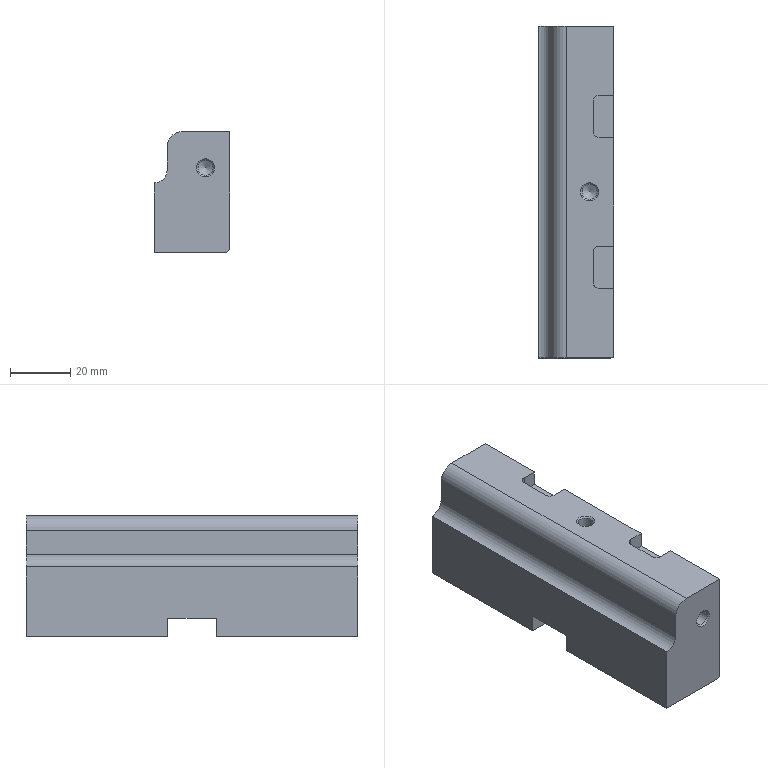Part | STEP file | gslz 2016.10.28-6_id746_x_t | 1 solid | 42 faces | box 25 x 110 x 40 mm | volume 96354 mm3 | plane 21 | cylinder 11 | cone 10 | commonest cylinder face diameters 4 x4 5 x3 6.8 x2 8.5 x1 10 x1
STEP:
#1=CARTESIAN_POINT('',(115.2,175.,53.));
#2=VERTEX_POINT('',#1);
#3=CARTESIAN_POINT('',(115.2,175.,57.));
#4=DIRECTION('',(1.,0.,0.));
#5=DIRECTION('',(0.,0.,-1.));
#6=AXIS2_PLACEMENT_3D('',#3,#4,#5);
#7=CIRCLE('',#6,4.);
#8=EDGE_CURVE('',#2,#2,#7,.T.);
#9=ORIENTED_EDGE('',*,*,#8,.F.);
#10=EDGE_LOOP('',(#9));
#11=FACE_BOUND('',#10,.T.);
#12=CARTESIAN_POINT('',(115.2,158.,40.));
#13=VERTEX_POINT('',#12);
#14=CARTESIAN_POINT('',(115.2,158.,45.));
#15=VERTEX_POINT('',#14);
#16=CARTESIAN_POINT('',(115.2,158.,35.));
#17=DIRECTION('',(0.,0.,1.));
#18=VECTOR('',#17,1.);
#19=LINE('',#16,#18);
#20=EDGE_CURVE('',#13,#15,#19,.T.);
#21=ORIENTED_EDGE('',*,*,#20,.F.);
#22=CARTESIAN_POINT('',(115.2,205.01,40.));
#23=VERTEX_POINT('',#22);
#24=CARTESIAN_POINT('',(115.2,930.778,40.));
#25=DIRECTION('',(0.,1.,0.));
#26=VECTOR('',#25,1.);
#27=LINE('',#24,#26);
#28=EDGE_CURVE('',#13,#23,#27,.T.);
#29=ORIENTED_EDGE('',*,*,#28,.T.);
#30=CARTESIAN_POINT('',(115.2,205.01,79.));
#31=VERTEX_POINT('',#30);
#32=CARTESIAN_POINT('',(115.2,205.01,79.));
#33=DIRECTION('',(0.,0.,-1.));
#34=VECTOR('',#33,1.);
#35=LINE('',#32,#34);
#36=EDGE_CURVE('',#31,#23,#35,.T.);
#37=ORIENTED_EDGE('',*,*,#36,.F.);
#38=CARTESIAN_POINT('',(115.2,182.,79.));
#39=VERTEX_POINT('',#38);
#40=CARTESIAN_POINT('',(115.2,101.,79.));
#41=DIRECTION('',(0.,1.,0.));
#42=VECTOR('',#41,1.);
#43=LINE('',#40,#42);
#44=EDGE_CURVE('',#39,#31,#43,.T.);
#45=ORIENTED_EDGE('',*,*,#44,.F.);
#46=CARTESIAN_POINT('',(115.2,182.,74.));
#47=VERTEX_POINT('',#46);
#48=CARTESIAN_POINT('',(115.2,182.,49.));
#49=DIRECTION('',(0.,-0.000000014,-1.));
#50=VECTOR('',#49,1.);
#51=LINE('',#48,#50);
#52=EDGE_CURVE('',#39,#47,#51,.T.);
#53=ORIENTED_EDGE('',*,*,#52,.T.);
#54=CARTESIAN_POINT('',(115.2,168.,74.));
#55=VERTEX_POINT('',#54);
#56=CARTESIAN_POINT('',(115.2,932.793,74.));
#57=DIRECTION('',(0.,1.,0.000000015));
#58=VECTOR('',#57,1.);
#59=LINE('',#56,#58);
#60=EDGE_CURVE('',#55,#47,#59,.T.);
#61=ORIENTED_EDGE('',*,*,#60,.F.);
#62=CARTESIAN_POINT('',(115.2,168.,79.));
#63=VERTEX_POINT('',#62);
#64=CARTESIAN_POINT('',(115.2,168.,49.));
#65=DIRECTION('',(0.,-0.000000014,-1.));
#66=VECTOR('',#65,1.);
#67=LINE('',#64,#66);
#68=EDGE_CURVE('',#63,#55,#67,.T.);
#69=ORIENTED_EDGE('',*,*,#68,.F.);
#70=CARTESIAN_POINT('',(115.2,132.,79.));
#71=VERTEX_POINT('',#70);
#72=CARTESIAN_POINT('',(115.2,101.,79.));
#73=DIRECTION('',(0.,1.,0.));
#74=VECTOR('',#73,1.);
#75=LINE('',#72,#74);
#76=EDGE_CURVE('',#71,#63,#75,.T.);
#77=ORIENTED_EDGE('',*,*,#76,.F.);
#78=CARTESIAN_POINT('',(115.2,132.,74.));
#79=VERTEX_POINT('',#78);
#80=CARTESIAN_POINT('',(115.2,132.,49.));
#81=DIRECTION('',(0.,-0.000000014,-1.));
#82=VECTOR('',#81,1.);
#83=LINE('',#80,#82);
#84=EDGE_CURVE('',#71,#79,#83,.T.);
#85=ORIENTED_EDGE('',*,*,#84,.T.);
#86=CARTESIAN_POINT('',(115.2,118.,74.));
#87=VERTEX_POINT('',#86);
#88=CARTESIAN_POINT('',(115.2,928.763,74.));
#89=DIRECTION('',(0.,1.,-0.000000015));
#90=VECTOR('',#89,1.);
#91=LINE('',#88,#90);
#92=EDGE_CURVE('',#87,#79,#91,.T.);
#93=ORIENTED_EDGE('',*,*,#92,.F.);
#94=CARTESIAN_POINT('',(115.2,118.,79.));
#95=VERTEX_POINT('',#94);
#96=CARTESIAN_POINT('',(115.2,118.,49.));
#97=DIRECTION('',(0.,-0.000000014,-1.));
#98=VECTOR('',#97,1.);
#99=LINE('',#96,#98);
#100=EDGE_CURVE('',#95,#87,#99,.T.);
#101=ORIENTED_EDGE('',*,*,#100,.F.);
#102=CARTESIAN_POINT('',(115.2,95.01,79.));
#103=VERTEX_POINT('',#102);
#104=CARTESIAN_POINT('',(115.2,101.,79.));
#105=DIRECTION('',(0.,1.,0.));
#106=VECTOR('',#105,1.);
#107=LINE('',#104,#106);
#108=EDGE_CURVE('',#103,#95,#107,.T.);
#109=ORIENTED_EDGE('',*,*,#108,.F.);
#110=CARTESIAN_POINT('',(115.2,95.01,40.));
#111=VERTEX_POINT('',#110);
#112=CARTESIAN_POINT('',(115.2,95.01,79.));
#113=DIRECTION('',(0.,0.,1.));
#114=VECTOR('',#113,1.);
#115=LINE('',#112,#114);
#116=EDGE_CURVE('',#111,#103,#115,.T.);
#117=ORIENTED_EDGE('',*,*,#116,.F.);
#118=CARTESIAN_POINT('',(115.2,142.,40.));
#119=VERTEX_POINT('',#118);
#120=CARTESIAN_POINT('',(115.2,930.778,40.));
#121=DIRECTION('',(0.,1.,0.));
#122=VECTOR('',#121,1.);
#123=LINE('',#120,#122);
#124=EDGE_CURVE('',#111,#119,#123,.T.);
#125=ORIENTED_EDGE('',*,*,#124,.T.);
#126=CARTESIAN_POINT('',(115.2,142.,45.));
#127=VERTEX_POINT('',#126);
#128=CARTESIAN_POINT('',(115.2,142.,46.));
#129=DIRECTION('',(0.,0.,1.));
#130=VECTOR('',#129,1.);
#131=LINE('',#128,#130);
#132=EDGE_CURVE('',#119,#127,#131,.T.);
#133=ORIENTED_EDGE('',*,*,#132,.T.);
#134=CARTESIAN_POINT('',(115.2,930.778,45.));
#135=DIRECTION('',(0.,1.,0.));
#136=VECTOR('',#135,1.);
#137=LINE('',#134,#136);
#138=EDGE_CURVE('',#127,#15,#137,.T.);
#139=ORIENTED_EDGE('',*,*,#138,.T.);
#140=EDGE_LOOP('',(#21,#29,#37,#45,#53,#61,#69,#77,#85,#93,#101,#109,#117,#125,#133,#139));
#141=FACE_BOUND('',#140,.T.);
#142=CARTESIAN_POINT('',(115.2,125.,53.));
#143=VERTEX_POINT('',#142);
#144=CARTESIAN_POINT('',(115.2,125.,57.));
#145=DIRECTION('',(1.,0.,0.));
#146=DIRECTION('',(0.,0.,-1.));
#147=AXIS2_PLACEMENT_3D('',#144,#145,#146);
#148=CIRCLE('',#147,4.);
#149=EDGE_CURVE('',#143,#143,#148,.T.);
#150=ORIENTED_EDGE('',*,*,#149,.F.);
#151=EDGE_LOOP('',(#150));
#152=FACE_BOUND('',#151,.T.);
#153=CARTESIAN_POINT('',(115.2,930.778,49.));
#154=DIRECTION('',(-1.,0.,0.));
#155=DIRECTION('',(0.,0.,1.));
#156=AXIS2_PLACEMENT_3D('',#153,#154,#155);
#157=PLANE('',#156);
#158=ADVANCED_FACE('',(#11,#141,#152),#157,.F.);
#159=CARTESIAN_POINT('',(114.2,95.01,39.));
#160=VERTEX_POINT('',#159);
#161=CARTESIAN_POINT('',(90.2,95.01,39.));
#162=VERTEX_POINT('',#161);
#163=CARTESIAN_POINT('',(100.2,95.01,39.));
#164=DIRECTION('',(-1.,0.,0.));
#165=VECTOR('',#164,1.);
#166=LINE('',#163,#165);
#167=EDGE_CURVE('',#160,#162,#166,.T.);
#168=ORIENTED_EDGE('',*,*,#167,.F.);
#169=CARTESIAN_POINT('',(127.2,95.01,52.));
#170=DIRECTION('',(0.7071,0.,0.7071));
#171=VECTOR('',#170,1.);
#172=LINE('',#169,#171);
#173=EDGE_CURVE('',#160,#111,#172,.T.);
#174=ORIENTED_EDGE('',*,*,#173,.T.);
#175=ORIENTED_EDGE('',*,*,#116,.T.);
#176=CARTESIAN_POINT('',(99.45,95.01,79.));
#177=VERTEX_POINT('',#176);
#178=CARTESIAN_POINT('',(100.2,95.01,79.));
#179=DIRECTION('',(1.,0.,0.));
#180=VECTOR('',#179,1.);
#181=LINE('',#178,#180);
#182=EDGE_CURVE('',#177,#103,#181,.T.);
#183=ORIENTED_EDGE('',*,*,#182,.F.);
#184=CARTESIAN_POINT('',(94.45,95.01,74.));
#185=VERTEX_POINT('',#184);
#186=CARTESIAN_POINT('',(99.45,95.01,74.));
#187=DIRECTION('',(0.,1.,0.));
#188=DIRECTION('',(1.,0.,0.));
#189=AXIS2_PLACEMENT_3D('',#186,#187,#188);
#190=CIRCLE('',#189,5.);
#191=EDGE_CURVE('',#185,#177,#190,.T.);
#192=ORIENTED_EDGE('',*,*,#191,.F.);
#193=CARTESIAN_POINT('',(94.45,95.01,66.25));
#194=VERTEX_POINT('',#193);
#195=CARTESIAN_POINT('',(94.45,95.01,79.));
#196=DIRECTION('',(0.,0.,1.));
#197=VECTOR('',#196,1.);
#198=LINE('',#195,#197);
#199=EDGE_CURVE('',#194,#185,#198,.T.);
#200=ORIENTED_EDGE('',*,*,#199,.F.);
#201=CARTESIAN_POINT('',(90.2,95.01,62.));
#202=VERTEX_POINT('',#201);
#203=CARTESIAN_POINT('',(90.2,95.01,66.25));
#204=DIRECTION('',(0.,-1.,0.));
#205=DIRECTION('',(1.,0.,0.));
#206=AXIS2_PLACEMENT_3D('',#203,#204,#205);
#207=CIRCLE('',#206,4.25);
#208=EDGE_CURVE('',#202,#194,#207,.T.);
#209=ORIENTED_EDGE('',*,*,#208,.F.);
#210=CARTESIAN_POINT('',(90.2,95.01,79.));
#211=DIRECTION('',(0.,0.,1.));
#212=VECTOR('',#211,1.);
#213=LINE('',#210,#212);
#214=EDGE_CURVE('',#162,#202,#213,.T.);
#215=ORIENTED_EDGE('',*,*,#214,.F.);
#216=EDGE_LOOP('',(#168,#174,#175,#183,#192,#200,#209,#215));
#217=FACE_BOUND('',#216,.T.);
#218=CARTESIAN_POINT('',(110.2,95.01,67.));
#219=VERTEX_POINT('',#218);
#220=CARTESIAN_POINT('',(107.2,95.01,67.));
#221=DIRECTION('',(0.,-1.,0.));
#222=DIRECTION('',(1.,0.,0.));
#223=AXIS2_PLACEMENT_3D('',#220,#221,#222);
#224=CIRCLE('',#223,3.);
#225=EDGE_CURVE('',#219,#219,#224,.T.);
#226=ORIENTED_EDGE('',*,*,#225,.F.);
#227=EDGE_LOOP('',(#226));
#228=FACE_BOUND('',#227,.T.);
#229=CARTESIAN_POINT('',(100.2,95.01,79.));
#230=DIRECTION('',(0.,1.,0.));
#231=DIRECTION('',(0.000000244,0.,-1.));
#232=AXIS2_PLACEMENT_3D('',#229,#230,#231);
#233=PLANE('',#232);
#234=ADVANCED_FACE('',(#217,#228),#233,.F.);
#235=CARTESIAN_POINT('',(110.402,182.,73.999));
#236=VERTEX_POINT('',#235);
#237=CARTESIAN_POINT('',(114.858,182.,74.));
#238=DIRECTION('',(1.,-0.000004636,0.0001633));
#239=VECTOR('',#238,1.);
#240=LINE('',#237,#239);
#241=EDGE_CURVE('',#236,#47,#240,.T.);
#242=ORIENTED_EDGE('',*,*,#241,.F.);
#243=CARTESIAN_POINT('',(108.402,180.,73.999));
#244=VERTEX_POINT('',#243);
#245=CARTESIAN_POINT('',(110.402,180.,73.999));
#246=DIRECTION('',(0.0001633,-0.000000015,-1.));
#247=DIRECTION('',(1.,-0.000004636,0.0001633));
#248=AXIS2_PLACEMENT_3D('',#245,#246,#247);
#249=ELLIPSE('',#248,2.,2.);
#250=EDGE_CURVE('',#244,#236,#249,.T.);
#251=ORIENTED_EDGE('',*,*,#250,.F.);
#252=CARTESIAN_POINT('',(108.402,170.,73.999));
#253=VERTEX_POINT('',#252);
#254=CARTESIAN_POINT('',(108.402,169.,73.999));
#255=DIRECTION('',(-0.000004439,-1.,0.000000014));
#256=VECTOR('',#255,1.);
#257=LINE('',#254,#256);
#258=EDGE_CURVE('',#244,#253,#257,.T.);
#259=ORIENTED_EDGE('',*,*,#258,.T.);
#260=CARTESIAN_POINT('',(110.402,168.,73.999));
#261=VERTEX_POINT('',#260);
#262=CARTESIAN_POINT('',(110.402,170.,73.999));
#263=DIRECTION('',(0.0001633,-0.000000015,-1.));
#264=DIRECTION('',(1.,-0.000004636,0.0001633));
#265=AXIS2_PLACEMENT_3D('',#262,#263,#264);
#266=ELLIPSE('',#265,2.,2.);
#267=EDGE_CURVE('',#261,#253,#266,.T.);
#268=ORIENTED_EDGE('',*,*,#267,.F.);
#269=CARTESIAN_POINT('',(114.858,168.,74.));
#270=DIRECTION('',(1.,-0.000004636,0.0001633));
#271=VECTOR('',#270,1.);
#272=LINE('',#269,#271);
#273=EDGE_CURVE('',#261,#55,#272,.T.);
#274=ORIENTED_EDGE('',*,*,#273,.T.);
#275=ORIENTED_EDGE('',*,*,#60,.T.);
#276=EDGE_LOOP('',(#242,#251,#259,#268,#274,#275));
#277=FACE_OUTER_BOUND('',#276,.T.);
#278=CARTESIAN_POINT('',(114.858,181.,74.));
#279=DIRECTION('',(0.0001633,0.000000015,-1.));
#280=DIRECTION('',(-1.,-0.000004636,-0.0001633));
#281=AXIS2_PLACEMENT_3D('',#278,#279,#280);
#282=PLANE('',#281);
#283=ADVANCED_FACE('',(#277),#282,.F.);
#284=ORIENTED_EDGE('',*,*,#241,.T.);
#285=ORIENTED_EDGE('',*,*,#52,.F.);
#286=CARTESIAN_POINT('',(110.401,182.,79.));
#287=VERTEX_POINT('',#286);
#288=CARTESIAN_POINT('',(90.2,182.,79.));
#289=DIRECTION('',(-1.,0.000004636,0.));
#290=VECTOR('',#289,1.);
#291=LINE('',#288,#290);
#292=EDGE_CURVE('',#39,#287,#291,.T.);
#293=ORIENTED_EDGE('',*,*,#292,.T.);
#294=CARTESIAN_POINT('',(110.402,182.,73.999));
#295=DIRECTION('',(-0.0002202,0.000000015,1.));
#296=VECTOR('',#295,1.);
#297=LINE('',#294,#296);
#298=EDGE_CURVE('',#236,#287,#297,.T.);
#299=ORIENTED_EDGE('',*,*,#298,.F.);
#300=EDGE_LOOP('',(#284,#285,#293,#299));
#301=FACE_OUTER_BOUND('',#300,.T.);
#302=CARTESIAN_POINT('',(114.858,182.,74.));
#303=DIRECTION('',(-0.000004636,-1.,0.000000014));
#304=DIRECTION('',(-1.,0.000004636,-0.0001633));
#305=AXIS2_PLACEMENT_3D('',#302,#303,#304);
#306=PLANE('',#305);
#307=ADVANCED_FACE('',(#301),#306,.T.);
#308=CARTESIAN_POINT('',(108.401,180.,79.));
#309=VERTEX_POINT('',#308);
#310=CARTESIAN_POINT('',(110.401,180.,79.));
#311=DIRECTION('',(0.,0.,-1.));
#312=DIRECTION('',(1.,-0.00006712,0.));
#313=AXIS2_PLACEMENT_3D('',#310,#311,#312);
#314=ELLIPSE('',#313,2.,2.);
#315=EDGE_CURVE('',#309,#287,#314,.T.);
#316=ORIENTED_EDGE('',*,*,#315,.F.);
#317=CARTESIAN_POINT('',(108.398,180.,91.473));
#318=DIRECTION('',(0.0002202,-0.000000015,-1.));
#319=VECTOR('',#318,1.);
#320=LINE('',#317,#319);
#321=EDGE_CURVE('',#309,#244,#320,.T.);
#322=ORIENTED_EDGE('',*,*,#321,.T.);
#323=ORIENTED_EDGE('',*,*,#250,.T.);
#324=ORIENTED_EDGE('',*,*,#298,.T.);
#325=EDGE_LOOP('',(#316,#322,#323,#324));
#326=FACE_OUTER_BOUND('',#325,.T.);
#327=CARTESIAN_POINT('',(110.398,180.,91.474));
#328=DIRECTION('',(0.0002202,-0.000000015,-1.));
#329=DIRECTION('',(-1.,0.,-0.0002202));
#330=AXIS2_PLACEMENT_3D('',#327,#328,#329);
#331=CYLINDRICAL_SURFACE('',#330,2.);
#332=ADVANCED_FACE('',(#326),#331,.F.);
#333=ORIENTED_EDGE('',*,*,#258,.F.);
#334=ORIENTED_EDGE('',*,*,#321,.F.);
#335=CARTESIAN_POINT('',(108.401,170.,79.));
#336=VERTEX_POINT('',#335);
#337=CARTESIAN_POINT('',(108.4,103.015,79.));
#338=DIRECTION('',(0.000004439,1.,0.));
#339=VECTOR('',#338,1.);
#340=LINE('',#337,#339);
#341=EDGE_CURVE('',#336,#309,#340,.T.);
#342=ORIENTED_EDGE('',*,*,#341,.F.);
#343=CARTESIAN_POINT('',(108.401,170.,79.));
#344=DIRECTION('',(-0.0002202,0.000000015,1.));
#345=VECTOR('',#344,1.);
#346=LINE('',#343,#345);
#347=EDGE_CURVE('',#253,#336,#346,.T.);
#348=ORIENTED_EDGE('',*,*,#347,.F.);
#349=EDGE_LOOP('',(#333,#334,#342,#348));
#350=FACE_OUTER_BOUND('',#349,.T.);
#351=CARTESIAN_POINT('',(108.397,-55.866,91.473));
#352=DIRECTION('',(-1.,0.000004439,-0.0002202));
#353=DIRECTION('',(-0.00001596,-0.9986,0.05234));
#354=AXIS2_PLACEMENT_3D('',#351,#352,#353);
#355=PLANE('',#354);
#356=ADVANCED_FACE('',(#350),#355,.F.);
#357=ORIENTED_EDGE('',*,*,#267,.T.);
#358=ORIENTED_EDGE('',*,*,#347,.T.);
#359=CARTESIAN_POINT('',(110.401,168.,79.));
#360=VERTEX_POINT('',#359);
#361=CARTESIAN_POINT('',(110.401,170.,79.));
#362=DIRECTION('',(0.,0.,-1.));
#363=DIRECTION('',(1.,-0.00006712,0.));
#364=AXIS2_PLACEMENT_3D('',#361,#362,#363);
#365=ELLIPSE('',#364,2.,2.);
#366=EDGE_CURVE('',#360,#336,#365,.T.);
#367=ORIENTED_EDGE('',*,*,#366,.F.);
#368=CARTESIAN_POINT('',(110.402,168.,73.999));
#369=DIRECTION('',(0.0002202,-0.000000015,-1.));
#370=VECTOR('',#369,1.);
#371=LINE('',#368,#370);
#372=EDGE_CURVE('',#360,#261,#371,.T.);
#373=ORIENTED_EDGE('',*,*,#372,.T.);
#374=EDGE_LOOP('',(#357,#358,#367,#373));
#375=FACE_OUTER_BOUND('',#374,.T.);
#376=CARTESIAN_POINT('',(110.398,170.,91.474));
#377=DIRECTION('',(0.0002202,-0.000000015,-1.));
#378=DIRECTION('',(-1.,0.,-0.0002202));
#379=AXIS2_PLACEMENT_3D('',#376,#377,#378);
#380=CYLINDRICAL_SURFACE('',#379,2.);
#381=ADVANCED_FACE('',(#375),#380,.F.);
#382=CARTESIAN_POINT('',(90.2,168.,79.));
#383=DIRECTION('',(-1.,0.000004636,0.));
#384=VECTOR('',#383,1.);
#385=LINE('',#382,#384);
#386=EDGE_CURVE('',#63,#360,#385,.T.);
#387=ORIENTED_EDGE('',*,*,#386,.F.);
#388=ORIENTED_EDGE('',*,*,#68,.T.);
#389=ORIENTED_EDGE('',*,*,#273,.F.);
#390=ORIENTED_EDGE('',*,*,#372,.F.);
#391=EDGE_LOOP('',(#387,#388,#389,#390));
#392=FACE_OUTER_BOUND('',#391,.T.);
#393=CARTESIAN_POINT('',(114.858,168.,74.));
#394=DIRECTION('',(-0.000004636,-1.,0.000000014));
#395=DIRECTION('',(-1.,0.000004636,-0.0001633));
#396=AXIS2_PLACEMENT_3D('',#393,#394,#395);
#397=PLANE('',#396);
#398=ADVANCED_FACE('',(#392),#397,.F.);
#399=CARTESIAN_POINT('',(114.2,205.01,39.));
#400=VERTEX_POINT('',#399);
#401=CARTESIAN_POINT('',(90.2,205.01,39.));
#402=VERTEX_POINT('',#401);
#403=CARTESIAN_POINT('',(100.2,205.01,39.));
#404=DIRECTION('',(-1.,0.000000182,0.));
#405=VECTOR('',#404,1.);
#406=LINE('',#403,#405);
#407=EDGE_CURVE('',#400,#402,#406,.T.);
#408=ORIENTED_EDGE('',*,*,#407,.F.);
#409=CARTESIAN_POINT('',(114.2,158.,39.));
#410=VERTEX_POINT('',#409);
#411=CARTESIAN_POINT('',(114.2,930.778,39.));
#412=DIRECTION('',(0.,-1.,0.));
#413=VECTOR('',#412,1.);
#414=LINE('',#411,#413);
#415=EDGE_CURVE('',#400,#410,#414,.T.);
#416=ORIENTED_EDGE('',*,*,#415,.T.);
#417=CARTESIAN_POINT('',(90.2,158.,39.));
#418=VERTEX_POINT('',#417);
#419=CARTESIAN_POINT('',(43.466,157.999,39.));
#420=DIRECTION('',(1.,0.0000204,0.));
#421=VECTOR('',#420,1.);
#422=LINE('',#419,#421);
#423=EDGE_CURVE('',#418,#410,#422,.T.);
#424=ORIENTED_EDGE('',*,*,#423,.F.);
#425=CARTESIAN_POINT('',(90.2,197.296,39.));
#426=DIRECTION('',(-0.00000015,-1.,0.));
#427=VECTOR('',#426,1.);
#428=LINE('',#425,#427);
#429=EDGE_CURVE('',#402,#418,#428,.T.);
#430=ORIENTED_EDGE('',*,*,#429,.F.);
#431=EDGE_LOOP('',(#408,#416,#424,#430));
#432=FACE_OUTER_BOUND('',#431,.T.);
#433=CARTESIAN_POINT('',(43.45,930.778,39.));
#434=DIRECTION('',(0.,0.,1.));
#435=DIRECTION('',(1.,0.,0.));
#436=AXIS2_PLACEMENT_3D('',#433,#434,#435);
#437=PLANE('',#436);
#438=ADVANCED_FACE('',(#432),#437,.F.);
#439=CARTESIAN_POINT('',(99.45,205.01,79.));
#440=VERTEX_POINT('',#439);
#441=CARTESIAN_POINT('',(94.45,205.01,74.));
#442=VERTEX_POINT('',#441);
#443=CARTESIAN_POINT('',(99.45,205.01,74.));
#444=DIRECTION('',(-0.000000182,-1.,0.));
#445=DIRECTION('',(-1.,0.000000182,0.));
#446=AXIS2_PLACEMENT_3D('',#443,#444,#445);
#447=CIRCLE('',#446,5.);
#448=EDGE_CURVE('',#440,#442,#447,.T.);
#449=ORIENTED_EDGE('',*,*,#448,.T.);
#450=CARTESIAN_POINT('',(94.45,150.,74.));
#451=DIRECTION('',(0.,-1.,0.));
#452=VECTOR('',#451,1.);
#453=LINE('',#450,#452);
#454=EDGE_CURVE('',#442,#185,#453,.T.);
#455=ORIENTED_EDGE('',*,*,#454,.T.);
#456=ORIENTED_EDGE('',*,*,#191,.T.);
#457=CARTESIAN_POINT('',(99.45,101.,79.));
#458=DIRECTION('',(0.,1.,0.));
#459=VECTOR('',#458,1.);
#460=LINE('',#457,#459);
#461=EDGE_CURVE('',#177,#440,#460,.T.);
#462=ORIENTED_EDGE('',*,*,#461,.T.);
#463=EDGE_LOOP('',(#449,#455,#456,#462));
#464=FACE_OUTER_BOUND('',#463,.T.);
#465=CARTESIAN_POINT('',(99.45,150.,74.));
#466=DIRECTION('',(0.,-1.,0.));
#467=DIRECTION('',(1.,0.,0.));
#468=AXIS2_PLACEMENT_3D('',#465,#466,#467);
#469=CYLINDRICAL_SURFACE('',#468,5.);
#470=ADVANCED_FACE('',(#464),#469,.T.);
#471=CARTESIAN_POINT('',(94.45,205.01,66.25));
#472=VERTEX_POINT('',#471);
#473=CARTESIAN_POINT('',(94.45,205.01,64.742));
#474=DIRECTION('',(0.,0.,1.));
#475=VECTOR('',#474,1.);
#476=LINE('',#473,#475);
#477=EDGE_CURVE('',#472,#442,#476,.T.);
#478=ORIENTED_EDGE('',*,*,#477,.F.);
#479=CARTESIAN_POINT('',(94.45,150.,66.25));
#480=DIRECTION('',(0.,1.,0.));
#481=VECTOR('',#480,1.);
#482=LINE('',#479,#481);
#483=EDGE_CURVE('',#194,#472,#482,.T.);
#484=ORIENTED_EDGE('',*,*,#483,.F.);
#485=ORIENTED_EDGE('',*,*,#199,.T.);
#486=ORIENTED_EDGE('',*,*,#454,.F.);
#487=EDGE_LOOP('',(#478,#484,#485,#486));
#488=FACE_OUTER_BOUND('',#487,.T.);
#489=CARTESIAN_POINT('',(94.45,150.,64.742));
#490=DIRECTION('',(-1.,0.,0.));
#491=DIRECTION('',(0.,0.,1.));
#492=AXIS2_PLACEMENT_3D('',#489,#490,#491);
#493=PLANE('',#492);
#494=ADVANCED_FACE('',(#488),#493,.T.);
#495=ORIENTED_EDGE('',*,*,#208,.T.);
#496=ORIENTED_EDGE('',*,*,#483,.T.);
#497=CARTESIAN_POINT('',(90.2,205.01,62.));
#498=VERTEX_POINT('',#497);
#499=CARTESIAN_POINT('',(90.2,205.01,66.25));
#500=DIRECTION('',(0.000000182,1.,0.));
#501=DIRECTION('',(-1.,0.000000182,0.));
#502=AXIS2_PLACEMENT_3D('',#499,#500,#501);
#503=CIRCLE('',#502,4.25);
#504=EDGE_CURVE('',#472,#498,#503,.T.);
#505=ORIENTED_EDGE('',*,*,#504,.T.);
#506=CARTESIAN_POINT('',(90.2,197.296,62.));
#507=DIRECTION('',(-0.00000015,-1.,0.));
#508=VECTOR('',#507,1.);
#509=LINE('',#506,#508);
#510=EDGE_CURVE('',#498,#202,#509,.T.);
#511=ORIENTED_EDGE('',*,*,#510,.T.);
#512=EDGE_LOOP('',(#495,#496,#505,#511));
#513=FACE_OUTER_BOUND('',#512,.T.);
#514=CARTESIAN_POINT('',(90.2,150.,66.25));
#515=DIRECTION('',(0.,-1.,0.));
#516=DIRECTION('',(1.,0.,0.));
#517=AXIS2_PLACEMENT_3D('',#514,#515,#516);
#518=CYLINDRICAL_SURFACE('',#517,4.25);
#519=ADVANCED_FACE('',(#513),#518,.F.);
#520=CARTESIAN_POINT('',(90.2,158.,45.));
#521=VERTEX_POINT('',#520);
#522=CARTESIAN_POINT('',(90.2,142.,45.));
#523=VERTEX_POINT('',#522);
#524=CARTESIAN_POINT('',(90.2,197.296,45.));
#525=DIRECTION('',(-0.00000015,-1.,0.));
#526=VECTOR('',#525,1.);
#527=LINE('',#524,#526);
#528=EDGE_CURVE('',#521,#523,#527,.T.);
#529=ORIENTED_EDGE('',*,*,#528,.T.);
#530=CARTESIAN_POINT('',(90.2,142.,39.));
#531=VERTEX_POINT('',#530);
#532=CARTESIAN_POINT('',(90.2,142.,60.492));
#533=DIRECTION('',(0.,0.,-1.));
#534=VECTOR('',#533,1.);
#535=LINE('',#532,#534);
#536=EDGE_CURVE('',#523,#531,#535,.T.);
#537=ORIENTED_EDGE('',*,*,#536,.T.);
#538=CARTESIAN_POINT('',(90.2,197.296,39.));
#539=DIRECTION('',(-0.00000015,-1.,0.));
#540=VECTOR('',#539,1.);
#541=LINE('',#538,#540);
#542=EDGE_CURVE('',#531,#162,#541,.T.);
#543=ORIENTED_EDGE('',*,*,#542,.T.);
#544=ORIENTED_EDGE('',*,*,#214,.T.);
#545=ORIENTED_EDGE('',*,*,#510,.F.);
#546=CARTESIAN_POINT('',(90.2,205.01,63.492));
#547=DIRECTION('',(0.,0.,1.));
#548=VECTOR('',#547,1.);
#549=LINE('',#546,#548);
#550=EDGE_CURVE('',#402,#498,#549,.T.);
#551=ORIENTED_EDGE('',*,*,#550,.F.);
#552=ORIENTED_EDGE('',*,*,#429,.T.);
#553=CARTESIAN_POINT('',(90.2,158.,35.));
#554=DIRECTION('',(0.,0.,-1.));
#555=VECTOR('',#554,1.);
#556=LINE('',#553,#555);
#557=EDGE_CURVE('',#521,#418,#556,.T.);
#558=ORIENTED_EDGE('',*,*,#557,.F.);
#559=EDGE_LOOP('',(#529,#537,#543,#544,#545,#551,#552,#558));
#560=FACE_OUTER_BOUND('',#559,.T.);
#561=CARTESIAN_POINT('',(90.2,197.296,63.492));
#562=DIRECTION('',(1.,-0.00000015,0.));
#563=DIRECTION('',(0.00000015,1.,0.));
#564=AXIS2_PLACEMENT_3D('',#561,#562,#563);
#565=PLANE('',#564);
#566=ADVANCED_FACE('',(#560),#565,.F.);
#567=ORIENTED_EDGE('',*,*,#36,.T.);
#568=CARTESIAN_POINT('',(127.2,205.01,52.));
#569=DIRECTION('',(-0.7071,0.000000129,-0.7071));
#570=VECTOR('',#569,1.);
#571=LINE('',#568,#570);
#572=EDGE_CURVE('',#23,#400,#571,.T.);
#573=ORIENTED_EDGE('',*,*,#572,.T.);
#574=ORIENTED_EDGE('',*,*,#407,.T.);
#575=ORIENTED_EDGE('',*,*,#550,.T.);
#576=ORIENTED_EDGE('',*,*,#504,.F.);
#577=ORIENTED_EDGE('',*,*,#477,.T.);
#578=ORIENTED_EDGE('',*,*,#448,.F.);
#579=CARTESIAN_POINT('',(100.2,205.01,79.));
#580=DIRECTION('',(-1.,0.000000182,0.));
#581=VECTOR('',#580,1.);
#582=LINE('',#579,#581);
#583=EDGE_CURVE('',#31,#440,#582,.T.);
#584=ORIENTED_EDGE('',*,*,#583,.F.);
#585=EDGE_LOOP('',(#567,#573,#574,#575,#576,#577,#578,#584));
#586=FACE_BOUND('',#585,.T.);
#587=CARTESIAN_POINT('',(110.2,205.01,67.));
#588=VERTEX_POINT('',#587);
#589=CARTESIAN_POINT('',(107.2,205.01,67.));
#590=DIRECTION('',(-0.000000365,-1.,0.));
#591=DIRECTION('',(1.,-0.000000365,0.));
#592=AXIS2_PLACEMENT_3D('',#589,#590,#591);
#593=CIRCLE('',#592,3.);
#594=EDGE_CURVE('',#588,#588,#593,.T.);
#595=ORIENTED_EDGE('',*,*,#594,.T.);
#596=EDGE_LOOP('',(#595));
#597=FACE_BOUND('',#596,.T.);
#598=CARTESIAN_POINT('',(100.2,205.01,79.));
#599=DIRECTION('',(-0.000000182,-1.,0.));
#600=DIRECTION('',(0.000000244,0.,-1.));
#601=AXIS2_PLACEMENT_3D('',#598,#599,#600);
#602=PLANE('',#601);
#603=ADVANCED_FACE('',(#586,#597),#602,.F.);
#604=CARTESIAN_POINT('',(110.2,150.,79.));
#605=VERTEX_POINT('',#604);
#606=CARTESIAN_POINT('',(107.2,150.,79.));
#607=DIRECTION('',(0.,0.,-1.));
#608=DIRECTION('',(1.,0.,0.));
#609=AXIS2_PLACEMENT_3D('',#606,#607,#608);
#610=CIRCLE('',#609,3.);
#611=EDGE_CURVE('',#605,#605,#610,.T.);
#612=ORIENTED_EDGE('',*,*,#611,.T.);
#613=EDGE_LOOP('',(#612));
#614=FACE_BOUND('',#613,.T.);
#615=ORIENTED_EDGE('',*,*,#386,.T.);
#616=ORIENTED_EDGE('',*,*,#366,.T.);
#617=ORIENTED_EDGE('',*,*,#341,.T.);
#618=ORIENTED_EDGE('',*,*,#315,.T.);
#619=ORIENTED_EDGE('',*,*,#292,.F.);
#620=ORIENTED_EDGE('',*,*,#44,.T.);
#621=ORIENTED_EDGE('',*,*,#583,.T.);
#622=ORIENTED_EDGE('',*,*,#461,.F.);
#623=ORIENTED_EDGE('',*,*,#182,.T.);
#624=ORIENTED_EDGE('',*,*,#108,.T.);
#625=CARTESIAN_POINT('',(110.401,118.,79.));
#626=VERTEX_POINT('',#625);
#627=CARTESIAN_POINT('',(114.858,118.,79.));
#628=DIRECTION('',(1.,-0.000004636,0.));
#629=VECTOR('',#628,1.);
#630=LINE('',#627,#629);
#631=EDGE_CURVE('',#626,#95,#630,.T.);
#632=ORIENTED_EDGE('',*,*,#631,.F.);
#633=CARTESIAN_POINT('',(108.401,120.,79.));
#634=VERTEX_POINT('',#633);
#635=CARTESIAN_POINT('',(110.401,120.,79.));
#636=DIRECTION('',(0.,0.,1.));
#637=DIRECTION('',(1.,-0.00006712,0.));
#638=AXIS2_PLACEMENT_3D('',#635,#636,#637);
#639=ELLIPSE('',#638,2.,2.);
#640=EDGE_CURVE('',#634,#626,#639,.T.);
#641=ORIENTED_EDGE('',*,*,#640,.F.);
#642=CARTESIAN_POINT('',(108.401,130.,79.));
#643=VERTEX_POINT('',#642);
#644=CARTESIAN_POINT('',(108.401,98.985,79.));
#645=DIRECTION('',(0.000004439,1.,0.));
#646=VECTOR('',#645,1.);
#647=LINE('',#644,#646);
#648=EDGE_CURVE('',#634,#643,#647,.T.);
#649=ORIENTED_EDGE('',*,*,#648,.T.);
#650=CARTESIAN_POINT('',(110.401,132.,79.));
#651=VERTEX_POINT('',#650);
#652=CARTESIAN_POINT('',(110.401,130.,79.));
#653=DIRECTION('',(0.,0.,1.));
#654=DIRECTION('',(1.,-0.00006712,0.));
#655=AXIS2_PLACEMENT_3D('',#652,#653,#654);
#656=ELLIPSE('',#655,2.,2.);
#657=EDGE_CURVE('',#651,#643,#656,.T.);
#658=ORIENTED_EDGE('',*,*,#657,.F.);
#659=CARTESIAN_POINT('',(114.858,132.,79.));
#660=DIRECTION('',(1.,-0.000004636,0.));
#661=VECTOR('',#660,1.);
#662=LINE('',#659,#661);
#663=EDGE_CURVE('',#651,#71,#662,.T.);
#664=ORIENTED_EDGE('',*,*,#663,.T.);
#665=ORIENTED_EDGE('',*,*,#76,.T.);
#666=EDGE_LOOP('',(#615,#616,#617,#618,#619,#620,#621,#622,#623,#624,#632,#641,#649,#658,#664,#665));
#667=FACE_BOUND('',#666,.T.);
#668=CARTESIAN_POINT('',(90.2,101.,79.));
#669=DIRECTION('',(0.,0.,1.));
#670=DIRECTION('',(1.,0.,0.));
#671=AXIS2_PLACEMENT_3D('',#668,#669,#670);
#672=PLANE('',#671);
#673=ADVANCED_FACE('',(#614,#667),#672,.T.);
#674=CARTESIAN_POINT('',(114.2,142.,39.));
#675=VERTEX_POINT('',#674);
#676=CARTESIAN_POINT('',(43.466,141.999,39.));
#677=DIRECTION('',(-1.,-0.0000204,0.));
#678=VECTOR('',#677,1.);
#679=LINE('',#676,#678);
#680=EDGE_CURVE('',#675,#531,#679,.T.);
#681=ORIENTED_EDGE('',*,*,#680,.F.);
#682=CARTESIAN_POINT('',(114.2,930.778,39.));
#683=DIRECTION('',(0.,-1.,0.));
#684=VECTOR('',#683,1.);
#685=LINE('',#682,#684);
#686=EDGE_CURVE('',#675,#160,#685,.T.);
#687=ORIENTED_EDGE('',*,*,#686,.T.);
#688=ORIENTED_EDGE('',*,*,#167,.T.);
#689=ORIENTED_EDGE('',*,*,#542,.F.);
#690=EDGE_LOOP('',(#681,#687,#688,#689));
#691=FACE_OUTER_BOUND('',#690,.T.);
#692=CARTESIAN_POINT('',(43.45,930.778,39.));
#693=DIRECTION('',(0.,0.,1.));
#694=DIRECTION('',(1.,0.,0.));
#695=AXIS2_PLACEMENT_3D('',#692,#693,#694);
#696=PLANE('',#695);
#697=ADVANCED_FACE('',(#691),#696,.F.);
#698=ORIENTED_EDGE('',*,*,#132,.F.);
#699=CARTESIAN_POINT('',(115.208,142.,40.008));
#700=DIRECTION('',(-0.7071,-0.00001443,-0.7071));
#701=VECTOR('',#700,1.);
#702=LINE('',#699,#701);
#703=EDGE_CURVE('',#119,#675,#702,.T.);
#704=ORIENTED_EDGE('',*,*,#703,.T.);
#705=ORIENTED_EDGE('',*,*,#680,.T.);
#706=ORIENTED_EDGE('',*,*,#536,.F.);
#707=CARTESIAN_POINT('',(102.7,142.,45.));
#708=DIRECTION('',(1.,0.0000204,0.));
#709=VECTOR('',#708,1.);
#710=LINE('',#707,#709);
#711=EDGE_CURVE('',#523,#127,#710,.T.);
#712=ORIENTED_EDGE('',*,*,#711,.T.);
#713=EDGE_LOOP('',(#698,#704,#705,#706,#712));
#714=FACE_OUTER_BOUND('',#713,.T.);
#715=CARTESIAN_POINT('',(102.7,142.,35.));
#716=DIRECTION('',(0.0000204,-1.,0.));
#717=DIRECTION('',(0.,0.,-1.));
#718=AXIS2_PLACEMENT_3D('',#715,#716,#717);
#719=PLANE('',#718);
#720=ADVANCED_FACE('',(#714),#719,.F.);
#721=ORIENTED_EDGE('',*,*,#423,.T.);
#722=CARTESIAN_POINT('',(115.208,158.,40.008));
#723=DIRECTION('',(0.7071,0.00001443,0.7071));
#724=VECTOR('',#723,1.);
#725=LINE('',#722,#724);
#726=EDGE_CURVE('',#410,#13,#725,.T.);
#727=ORIENTED_EDGE('',*,*,#726,.T.);
#728=ORIENTED_EDGE('',*,*,#20,.T.);
#729=CARTESIAN_POINT('',(102.7,158.,45.));
#730=DIRECTION('',(-1.,-0.0000204,0.));
#731=VECTOR('',#730,1.);
#732=LINE('',#729,#731);
#733=EDGE_CURVE('',#15,#521,#732,.T.);
#734=ORIENTED_EDGE('',*,*,#733,.T.);
#735=ORIENTED_EDGE('',*,*,#557,.T.);
#736=EDGE_LOOP('',(#721,#727,#728,#734,#735));
#737=FACE_OUTER_BOUND('',#736,.T.);
#738=CARTESIAN_POINT('',(102.7,158.,35.));
#739=DIRECTION('',(-0.0000204,1.,0.));
#740=DIRECTION('',(0.,0.,1.));
#741=AXIS2_PLACEMENT_3D('',#738,#739,#740);
#742=PLANE('',#741);
#743=ADVANCED_FACE('',(#737),#742,.F.);
#744=ORIENTED_EDGE('',*,*,#733,.F.);
#745=ORIENTED_EDGE('',*,*,#138,.F.);
#746=ORIENTED_EDGE('',*,*,#711,.F.);
#747=ORIENTED_EDGE('',*,*,#528,.F.);
#748=EDGE_LOOP('',(#744,#745,#746,#747));
#749=FACE_OUTER_BOUND('',#748,.T.);
#750=CARTESIAN_POINT('',(102.7,150.,45.));
#751=DIRECTION('',(0.,0.,1.));
#752=DIRECTION('',(0.0000204,-1.,0.));
#753=AXIS2_PLACEMENT_3D('',#750,#751,#752);
#754=PLANE('',#753);
#755=ADVANCED_FACE('',(#749),#754,.F.);
#756=CARTESIAN_POINT('',(110.402,118.,73.999));
#757=VERTEX_POINT('',#756);
#758=CARTESIAN_POINT('',(114.858,118.,74.));
#759=DIRECTION('',(1.,-0.000004636,0.0001633));
#760=VECTOR('',#759,1.);
#761=LINE('',#758,#760);
#762=EDGE_CURVE('',#757,#87,#761,.T.);
#763=ORIENTED_EDGE('',*,*,#762,.T.);
#764=ORIENTED_EDGE('',*,*,#92,.T.);
#765=CARTESIAN_POINT('',(110.402,132.,73.999));
#766=VERTEX_POINT('',#765);
#767=CARTESIAN_POINT('',(114.858,132.,74.));
#768=DIRECTION('',(-1.,0.000004636,-0.0001633));
#769=VECTOR('',#768,1.);
#770=LINE('',#767,#769);
#771=EDGE_CURVE('',#79,#766,#770,.T.);
#772=ORIENTED_EDGE('',*,*,#771,.T.);
#773=CARTESIAN_POINT('',(108.402,130.,73.999));
#774=VERTEX_POINT('',#773);
#775=CARTESIAN_POINT('',(110.402,130.,73.999));
#776=DIRECTION('',(0.0001633,-0.000000015,-1.));
#777=DIRECTION('',(1.,-0.000004636,0.0001633));
#778=AXIS2_PLACEMENT_3D('',#775,#776,#777);
#779=ELLIPSE('',#778,2.,2.);
#780=EDGE_CURVE('',#774,#766,#779,.T.);
#781=ORIENTED_EDGE('',*,*,#780,.F.);
#782=CARTESIAN_POINT('',(108.402,120.,73.999));
#783=VERTEX_POINT('',#782);
#784=CARTESIAN_POINT('',(108.402,119.,73.999));
#785=DIRECTION('',(0.000004439,1.,-0.000000014));
#786=VECTOR('',#785,1.);
#787=LINE('',#784,#786);
#788=EDGE_CURVE('',#783,#774,#787,.T.);
#789=ORIENTED_EDGE('',*,*,#788,.F.);
#790=CARTESIAN_POINT('',(110.402,120.,73.999));
#791=DIRECTION('',(0.0001633,-0.000000015,-1.));
#792=DIRECTION('',(1.,-0.000004636,0.0001633));
#793=AXIS2_PLACEMENT_3D('',#790,#791,#792);
#794=ELLIPSE('',#793,2.,2.);
#795=EDGE_CURVE('',#757,#783,#794,.T.);
#796=ORIENTED_EDGE('',*,*,#795,.F.);
#797=EDGE_LOOP('',(#763,#764,#772,#781,#789,#796));
#798=FACE_OUTER_BOUND('',#797,.T.);
#799=CARTESIAN_POINT('',(114.858,119.,74.));
#800=DIRECTION('',(0.0001633,-0.000000015,-1.));
#801=DIRECTION('',(-1.,0.,-0.0001633));
#802=AXIS2_PLACEMENT_3D('',#799,#800,#801);
#803=PLANE('',#802);
#804=ADVANCED_FACE('',(#798),#803,.F.);
#805=ORIENTED_EDGE('',*,*,#631,.T.);
#806=ORIENTED_EDGE('',*,*,#100,.T.);
#807=ORIENTED_EDGE('',*,*,#762,.F.);
#808=CARTESIAN_POINT('',(110.402,118.,73.999));
#809=DIRECTION('',(0.0002202,-0.000000015,-1.));
#810=VECTOR('',#809,1.);
#811=LINE('',#808,#810);
#812=EDGE_CURVE('',#626,#757,#811,.T.);
#813=ORIENTED_EDGE('',*,*,#812,.F.);
#814=EDGE_LOOP('',(#805,#806,#807,#813));
#815=FACE_OUTER_BOUND('',#814,.T.);
#816=CARTESIAN_POINT('',(114.858,118.,74.));
#817=DIRECTION('',(-0.000004636,-1.,0.000000014));
#818=DIRECTION('',(-1.,0.000004636,-0.0001633));
#819=AXIS2_PLACEMENT_3D('',#816,#817,#818);
#820=PLANE('',#819);
#821=ADVANCED_FACE('',(#815),#820,.F.);
#822=ORIENTED_EDGE('',*,*,#771,.F.);
#823=ORIENTED_EDGE('',*,*,#84,.F.);
#824=ORIENTED_EDGE('',*,*,#663,.F.);
#825=CARTESIAN_POINT('',(110.402,132.,73.999));
#826=DIRECTION('',(-0.0002202,0.000000015,1.));
#827=VECTOR('',#826,1.);
#828=LINE('',#825,#827);
#829=EDGE_CURVE('',#766,#651,#828,.T.);
#830=ORIENTED_EDGE('',*,*,#829,.F.);
#831=EDGE_LOOP('',(#822,#823,#824,#830));
#832=FACE_OUTER_BOUND('',#831,.T.);
#833=CARTESIAN_POINT('',(114.858,132.,74.));
#834=DIRECTION('',(-0.000004636,-1.,0.000000014));
#835=DIRECTION('',(-1.,0.000004636,-0.0001633));
#836=AXIS2_PLACEMENT_3D('',#833,#834,#835);
#837=PLANE('',#836);
#838=ADVANCED_FACE('',(#832),#837,.T.);
#839=ORIENTED_EDGE('',*,*,#788,.T.);
#840=CARTESIAN_POINT('',(108.398,130.,91.473));
#841=DIRECTION('',(0.0002202,-0.000000015,-1.));
#842=VECTOR('',#841,1.);
#843=LINE('',#840,#842);
#844=EDGE_CURVE('',#643,#774,#843,.T.);
#845=ORIENTED_EDGE('',*,*,#844,.F.);
#846=ORIENTED_EDGE('',*,*,#648,.F.);
#847=CARTESIAN_POINT('',(108.401,120.,79.));
#848=DIRECTION('',(-0.0002202,0.000000015,1.));
#849=VECTOR('',#848,1.);
#850=LINE('',#847,#849);
#851=EDGE_CURVE('',#783,#634,#850,.T.);
#852=ORIENTED_EDGE('',*,*,#851,.F.);
#853=EDGE_LOOP('',(#839,#845,#846,#852));
#854=FACE_OUTER_BOUND('',#853,.T.);
#855=CARTESIAN_POINT('',(108.397,-105.866,91.473));
#856=DIRECTION('',(-1.,0.000004439,-0.0002202));
#857=DIRECTION('',(-0.00001596,-0.9986,0.05234));
#858=AXIS2_PLACEMENT_3D('',#855,#856,#857);
#859=PLANE('',#858);
#860=ADVANCED_FACE('',(#854),#859,.F.);
#861=ORIENTED_EDGE('',*,*,#795,.T.);
#862=ORIENTED_EDGE('',*,*,#851,.T.);
#863=ORIENTED_EDGE('',*,*,#640,.T.);
#864=ORIENTED_EDGE('',*,*,#812,.T.);
#865=EDGE_LOOP('',(#861,#862,#863,#864));
#866=FACE_OUTER_BOUND('',#865,.T.);
#867=CARTESIAN_POINT('',(110.398,120.,91.474));
#868=DIRECTION('',(0.0002202,-0.000000015,-1.));
#869=DIRECTION('',(-1.,0.,-0.0002202));
#870=AXIS2_PLACEMENT_3D('',#867,#868,#869);
#871=CYLINDRICAL_SURFACE('',#870,2.);
#872=ADVANCED_FACE('',(#866),#871,.F.);
#873=ORIENTED_EDGE('',*,*,#657,.T.);
#874=ORIENTED_EDGE('',*,*,#844,.T.);
#875=ORIENTED_EDGE('',*,*,#780,.T.);
#876=ORIENTED_EDGE('',*,*,#829,.T.);
#877=EDGE_LOOP('',(#873,#874,#875,#876));
#878=FACE_OUTER_BOUND('',#877,.T.);
#879=CARTESIAN_POINT('',(110.398,130.,91.474));
#880=DIRECTION('',(0.0002202,-0.000000015,-1.));
#881=DIRECTION('',(-1.,0.,-0.0002202));
#882=AXIS2_PLACEMENT_3D('',#879,#880,#881);
#883=CYLINDRICAL_SURFACE('',#882,2.);
#884=ADVANCED_FACE('',(#878),#883,.F.);
#885=CARTESIAN_POINT('',(104.7,95.51,67.));
#886=VERTEX_POINT('',#885);
#887=CARTESIAN_POINT('',(107.2,95.51,67.));
#888=DIRECTION('',(0.,1.,0.));
#889=DIRECTION('',(-1.,0.,0.));
#890=AXIS2_PLACEMENT_3D('',#887,#888,#889);
#891=CIRCLE('',#890,2.5);
#892=EDGE_CURVE('',#886,#886,#891,.T.);
#893=ORIENTED_EDGE('',*,*,#892,.T.);
#894=EDGE_LOOP('',(#893));
#895=FACE_BOUND('',#894,.T.);
#896=ORIENTED_EDGE('',*,*,#225,.T.);
#897=EDGE_LOOP('',(#896));
#898=FACE_BOUND('',#897,.T.);
#899=CARTESIAN_POINT('',(107.2,95.01,67.));
#900=DIRECTION('',(0.,-1.,0.));
#901=DIRECTION('',(1.,0.,0.));
#902=AXIS2_PLACEMENT_3D('',#899,#900,#901);
#903=CONICAL_SURFACE('',#902,3.,45.);
#904=ADVANCED_FACE('',(#895,#898),#903,.F.);
#905=CARTESIAN_POINT('',(109.7,110.01,67.));
#906=VERTEX_POINT('',#905);
#907=CARTESIAN_POINT('',(107.2,110.01,67.));
#908=DIRECTION('',(0.,1.,0.));
#909=DIRECTION('',(1.,0.,0.));
#910=AXIS2_PLACEMENT_3D('',#907,#908,#909);
#911=CIRCLE('',#910,2.5);
#912=EDGE_CURVE('',#906,#906,#911,.T.);
#913=ORIENTED_EDGE('',*,*,#912,.F.);
#914=EDGE_LOOP('',(#913));
#915=FACE_BOUND('',#914,.T.);
#916=CARTESIAN_POINT('',(107.2,111.512,67.));
#917=VERTEX_POINT('',#916);
#918=VERTEX_LOOP('',#917);
#919=FACE_BOUND('',#918,.T.);
#920=CARTESIAN_POINT('',(107.2,110.01,67.));
#921=DIRECTION('',(0.,-1.,0.));
#922=DIRECTION('',(-1.,0.,0.));
#923=AXIS2_PLACEMENT_3D('',#920,#921,#922);
#924=CONICAL_SURFACE('',#923,2.5,59.);
#925=ADVANCED_FACE('',(#915,#919),#924,.F.);
#926=ORIENTED_EDGE('',*,*,#912,.T.);
#927=EDGE_LOOP('',(#926));
#928=FACE_BOUND('',#927,.T.);
#929=ORIENTED_EDGE('',*,*,#892,.F.);
#930=EDGE_LOOP('',(#929));
#931=FACE_BOUND('',#930,.T.);
#932=CARTESIAN_POINT('',(107.2,95.01,67.));
#933=DIRECTION('',(0.,1.,0.));
#934=DIRECTION('',(-1.,0.,0.));
#935=AXIS2_PLACEMENT_3D('',#932,#933,#934);
#936=CYLINDRICAL_SURFACE('',#935,2.5);
#937=ADVANCED_FACE('',(#928,#931),#936,.F.);
#938=CARTESIAN_POINT('',(104.7,204.51,67.));
#939=VERTEX_POINT('',#938);
#940=CARTESIAN_POINT('',(107.2,204.51,67.));
#941=DIRECTION('',(0.000000365,1.,0.));
#942=DIRECTION('',(-1.,0.000000365,0.));
#943=AXIS2_PLACEMENT_3D('',#940,#941,#942);
#944=CIRCLE('',#943,2.5);
#945=EDGE_CURVE('',#939,#939,#944,.T.);
#946=ORIENTED_EDGE('',*,*,#945,.F.);
#947=EDGE_LOOP('',(#946));
#948=FACE_BOUND('',#947,.T.);
#949=ORIENTED_EDGE('',*,*,#594,.F.);
#950=EDGE_LOOP('',(#949));
#951=FACE_BOUND('',#950,.T.);
#952=CARTESIAN_POINT('',(107.2,205.01,67.));
#953=DIRECTION('',(0.000000365,1.,0.));
#954=DIRECTION('',(1.,-0.000000365,0.));
#955=AXIS2_PLACEMENT_3D('',#952,#953,#954);
#956=CONICAL_SURFACE('',#955,3.,45.);
#957=ADVANCED_FACE('',(#948,#951),#956,.F.);
#958=CARTESIAN_POINT('',(109.7,190.01,67.));
#959=VERTEX_POINT('',#958);
#960=CARTESIAN_POINT('',(107.2,190.01,67.));
#961=DIRECTION('',(0.000000365,1.,0.));
#962=DIRECTION('',(1.,-0.000000365,0.));
#963=AXIS2_PLACEMENT_3D('',#960,#961,#962);
#964=CIRCLE('',#963,2.5);
#965=EDGE_CURVE('',#959,#959,#964,.T.);
#966=ORIENTED_EDGE('',*,*,#965,.T.);
#967=EDGE_LOOP('',(#966));
#968=FACE_BOUND('',#967,.T.);
#969=CARTESIAN_POINT('',(107.2,188.508,67.));
#970=VERTEX_POINT('',#969);
#971=VERTEX_LOOP('',#970);
#972=FACE_BOUND('',#971,.T.);
#973=CARTESIAN_POINT('',(107.2,190.01,67.));
#974=DIRECTION('',(0.000000365,1.,0.));
#975=DIRECTION('',(-1.,0.000000365,0.));
#976=AXIS2_PLACEMENT_3D('',#973,#974,#975);
#977=CONICAL_SURFACE('',#976,2.5,59.);
#978=ADVANCED_FACE('',(#968,#972),#977,.F.);
#979=ORIENTED_EDGE('',*,*,#965,.F.);
#980=EDGE_LOOP('',(#979));
#981=FACE_BOUND('',#980,.T.);
#982=ORIENTED_EDGE('',*,*,#945,.T.);
#983=EDGE_LOOP('',(#982));
#984=FACE_BOUND('',#983,.T.);
#985=CARTESIAN_POINT('',(107.2,205.01,67.));
#986=DIRECTION('',(-0.000000365,-1.,0.));
#987=DIRECTION('',(1.,-0.000000365,0.));
#988=AXIS2_PLACEMENT_3D('',#985,#986,#987);
#989=CYLINDRICAL_SURFACE('',#988,2.5);
#990=ADVANCED_FACE('',(#981,#984),#989,.F.);
#991=CARTESIAN_POINT('',(114.6,175.,60.4));
#992=VERTEX_POINT('',#991);
#993=CARTESIAN_POINT('',(114.6,175.,57.));
#994=DIRECTION('',(1.,0.,0.));
#995=DIRECTION('',(0.,0.,1.));
#996=AXIS2_PLACEMENT_3D('',#993,#994,#995);
#997=CIRCLE('',#996,3.4);
#998=EDGE_CURVE('',#992,#992,#997,.T.);
#999=ORIENTED_EDGE('',*,*,#998,.F.);
#1000=EDGE_LOOP('',(#999));
#1001=FACE_BOUND('',#1000,.T.);
#1002=ORIENTED_EDGE('',*,*,#8,.T.);
#1003=EDGE_LOOP('',(#1002));
#1004=FACE_BOUND('',#1003,.T.);
#1005=CARTESIAN_POINT('',(115.2,175.,57.));
#1006=DIRECTION('',(1.,0.,0.));
#1007=DIRECTION('',(0.,0.,-1.));
#1008=AXIS2_PLACEMENT_3D('',#1005,#1006,#1007);
#1009=CONICAL_SURFACE('',#1008,4.,45.);
#1010=ADVANCED_FACE('',(#1001,#1004),#1009,.F.);
#1011=CARTESIAN_POINT('',(98.2,175.,53.6));
#1012=VERTEX_POINT('',#1011);
#1013=CARTESIAN_POINT('',(98.2,175.,57.));
#1014=DIRECTION('',(-1.,0.,0.));
#1015=DIRECTION('',(0.,0.,-1.));
#1016=AXIS2_PLACEMENT_3D('',#1013,#1014,#1015);
#1017=CIRCLE('',#1016,3.4);
#1018=EDGE_CURVE('',#1012,#1012,#1017,.T.);
#1019=ORIENTED_EDGE('',*,*,#1018,.T.);
#1020=EDGE_LOOP('',(#1019));
#1021=FACE_BOUND('',#1020,.T.);
#1022=ORIENTED_EDGE('',*,*,#998,.T.);
#1023=EDGE_LOOP('',(#1022));
#1024=FACE_BOUND('',#1023,.T.);
#1025=CARTESIAN_POINT('',(115.2,175.,57.));
#1026=DIRECTION('',(-1.,0.,0.));
#1027=DIRECTION('',(0.,-1.,0.));
#1028=AXIS2_PLACEMENT_3D('',#1025,#1026,#1027);
#1029=CYLINDRICAL_SURFACE('',#1028,3.4);
#1030=ADVANCED_FACE('',(#1021,#1024),#1029,.F.);
#1031=ORIENTED_EDGE('',*,*,#1018,.F.);
#1032=EDGE_LOOP('',(#1031));
#1033=FACE_BOUND('',#1032,.T.);
#1034=CARTESIAN_POINT('',(96.157,175.,57.));
#1035=VERTEX_POINT('',#1034);
#1036=VERTEX_LOOP('',#1035);
#1037=FACE_BOUND('',#1036,.T.);
#1038=CARTESIAN_POINT('',(98.2,175.,57.));
#1039=DIRECTION('',(1.,0.,0.));
#1040=DIRECTION('',(0.,0.,1.));
#1041=AXIS2_PLACEMENT_3D('',#1038,#1039,#1040);
#1042=CONICAL_SURFACE('',#1041,3.4,59.);
#1043=ADVANCED_FACE('',(#1033,#1037),#1042,.F.);
#1044=CARTESIAN_POINT('',(114.6,125.,60.4));
#1045=VERTEX_POINT('',#1044);
#1046=CARTESIAN_POINT('',(114.6,125.,57.));
#1047=DIRECTION('',(1.,0.,0.));
#1048=DIRECTION('',(0.,0.,1.));
#1049=AXIS2_PLACEMENT_3D('',#1046,#1047,#1048);
#1050=CIRCLE('',#1049,3.4);
#1051=EDGE_CURVE('',#1045,#1045,#1050,.T.);
#1052=ORIENTED_EDGE('',*,*,#1051,.F.);
#1053=EDGE_LOOP('',(#1052));
#1054=FACE_BOUND('',#1053,.T.);
#1055=ORIENTED_EDGE('',*,*,#149,.T.);
#1056=EDGE_LOOP('',(#1055));
#1057=FACE_BOUND('',#1056,.T.);
#1058=CARTESIAN_POINT('',(115.2,125.,57.));
#1059=DIRECTION('',(1.,0.,0.));
#1060=DIRECTION('',(0.,0.,-1.));
#1061=AXIS2_PLACEMENT_3D('',#1058,#1059,#1060);
#1062=CONICAL_SURFACE('',#1061,4.,45.);
#1063=ADVANCED_FACE('',(#1054,#1057),#1062,.F.);
#1064=CARTESIAN_POINT('',(98.2,125.,53.6));
#1065=VERTEX_POINT('',#1064);
#1066=CARTESIAN_POINT('',(98.2,125.,57.));
#1067=DIRECTION('',(-1.,0.,0.));
#1068=DIRECTION('',(0.,0.,-1.));
#1069=AXIS2_PLACEMENT_3D('',#1066,#1067,#1068);
#1070=CIRCLE('',#1069,3.4);
#1071=EDGE_CURVE('',#1065,#1065,#1070,.T.);
#1072=ORIENTED_EDGE('',*,*,#1071,.T.);
#1073=EDGE_LOOP('',(#1072));
#1074=FACE_BOUND('',#1073,.T.);
#1075=ORIENTED_EDGE('',*,*,#1051,.T.);
#1076=EDGE_LOOP('',(#1075));
#1077=FACE_BOUND('',#1076,.T.);
#1078=CARTESIAN_POINT('',(115.2,125.,57.));
#1079=DIRECTION('',(-1.,0.,0.));
#1080=DIRECTION('',(0.,-1.,0.));
#1081=AXIS2_PLACEMENT_3D('',#1078,#1079,#1080);
#1082=CYLINDRICAL_SURFACE('',#1081,3.4);
#1083=ADVANCED_FACE('',(#1074,#1077),#1082,.F.);
#1084=ORIENTED_EDGE('',*,*,#1071,.F.);
#1085=EDGE_LOOP('',(#1084));
#1086=FACE_BOUND('',#1085,.T.);
#1087=CARTESIAN_POINT('',(96.157,125.,57.));
#1088=VERTEX_POINT('',#1087);
#1089=VERTEX_LOOP('',#1088);
#1090=FACE_BOUND('',#1089,.T.);
#1091=CARTESIAN_POINT('',(98.2,125.,57.));
#1092=DIRECTION('',(1.,0.,0.));
#1093=DIRECTION('',(0.,0.,1.));
#1094=AXIS2_PLACEMENT_3D('',#1091,#1092,#1093);
#1095=CONICAL_SURFACE('',#1094,3.4,59.);
#1096=ADVANCED_FACE('',(#1086,#1090),#1095,.F.);
#1097=ORIENTED_EDGE('',*,*,#726,.F.);
#1098=ORIENTED_EDGE('',*,*,#415,.F.);
#1099=ORIENTED_EDGE('',*,*,#572,.F.);
#1100=ORIENTED_EDGE('',*,*,#28,.F.);
#1101=EDGE_LOOP('',(#1097,#1098,#1099,#1100));
#1102=FACE_OUTER_BOUND('',#1101,.T.);
#1103=CARTESIAN_POINT('',(115.2,930.778,40.));
#1104=DIRECTION('',(-0.7071,0.,0.7071));
#1105=DIRECTION('',(0.,-1.,0.));
#1106=AXIS2_PLACEMENT_3D('',#1103,#1104,#1105);
#1107=PLANE('',#1106);
#1108=ADVANCED_FACE('',(#1102),#1107,.F.);
#1109=ORIENTED_EDGE('',*,*,#173,.F.);
#1110=ORIENTED_EDGE('',*,*,#686,.F.);
#1111=ORIENTED_EDGE('',*,*,#703,.F.);
#1112=ORIENTED_EDGE('',*,*,#124,.F.);
#1113=EDGE_LOOP('',(#1109,#1110,#1111,#1112));
#1114=FACE_OUTER_BOUND('',#1113,.T.);
#1115=CARTESIAN_POINT('',(115.2,930.778,40.));
#1116=DIRECTION('',(-0.7071,0.,0.7071));
#1117=DIRECTION('',(0.7071,0.,0.7071));
#1118=AXIS2_PLACEMENT_3D('',#1115,#1116,#1117);
#1119=PLANE('',#1118);
#1120=ADVANCED_FACE('',(#1114),#1119,.F.);
#1121=CARTESIAN_POINT('',(104.7,150.,67.));
#1122=VERTEX_POINT('',#1121);
#1123=CARTESIAN_POINT('',(107.2,150.,67.));
#1124=DIRECTION('',(0.,0.,-1.));
#1125=DIRECTION('',(-1.,0.,0.));
#1126=AXIS2_PLACEMENT_3D('',#1123,#1124,#1125);
#1127=CIRCLE('',#1126,2.5);
#1128=EDGE_CURVE('',#1122,#1122,#1127,.T.);
#1129=ORIENTED_EDGE('',*,*,#1128,.F.);
#1130=EDGE_LOOP('',(#1129));
#1131=FACE_BOUND('',#1130,.T.);
#1132=CARTESIAN_POINT('',(107.2,150.,65.498));
#1133=VERTEX_POINT('',#1132);
#1134=VERTEX_LOOP('',#1133);
#1135=FACE_BOUND('',#1134,.T.);
#1136=CARTESIAN_POINT('',(107.2,150.,67.));
#1137=DIRECTION('',(0.,0.,1.));
#1138=DIRECTION('',(1.,0.,0.));
#1139=AXIS2_PLACEMENT_3D('',#1136,#1137,#1138);
#1140=CONICAL_SURFACE('',#1139,2.5,59.);
#1141=ADVANCED_FACE('',(#1131,#1135),#1140,.F.);
#1142=CARTESIAN_POINT('',(109.7,150.,78.5));
#1143=VERTEX_POINT('',#1142);
#1144=CARTESIAN_POINT('',(107.2,150.,78.5));
#1145=DIRECTION('',(0.,0.,1.));
#1146=DIRECTION('',(1.,0.,0.));
#1147=AXIS2_PLACEMENT_3D('',#1144,#1145,#1146);
#1148=CIRCLE('',#1147,2.5);
#1149=EDGE_CURVE('',#1143,#1143,#1148,.T.);
#1150=ORIENTED_EDGE('',*,*,#1149,.T.);
#1151=EDGE_LOOP('',(#1150));
#1152=FACE_BOUND('',#1151,.T.);
#1153=ORIENTED_EDGE('',*,*,#1128,.T.);
#1154=EDGE_LOOP('',(#1153));
#1155=FACE_BOUND('',#1154,.T.);
#1156=CARTESIAN_POINT('',(107.2,150.,79.));
#1157=DIRECTION('',(0.,0.,-1.));
#1158=DIRECTION('',(-1.,0.,0.));
#1159=AXIS2_PLACEMENT_3D('',#1156,#1157,#1158);
#1160=CYLINDRICAL_SURFACE('',#1159,2.5);
#1161=ADVANCED_FACE('',(#1152,#1155),#1160,.F.);
#1162=ORIENTED_EDGE('',*,*,#1149,.F.);
#1163=EDGE_LOOP('',(#1162));
#1164=FACE_BOUND('',#1163,.T.);
#1165=ORIENTED_EDGE('',*,*,#611,.F.);
#1166=EDGE_LOOP('',(#1165));
#1167=FACE_BOUND('',#1166,.T.);
#1168=CARTESIAN_POINT('',(107.2,150.,79.));
#1169=DIRECTION('',(0.,0.,1.));
#1170=DIRECTION('',(-1.,0.,0.));
#1171=AXIS2_PLACEMENT_3D('',#1168,#1169,#1170);
#1172=CONICAL_SURFACE('',#1171,3.,45.);
#1173=ADVANCED_FACE('',(#1164,#1167),#1172,.F.);
#1174=CLOSED_SHELL('',(#158,#234,#283,#307,#332,#356,#381,#398,#438,#470,#494,#519,#566,#603,#673,#697,#720,#743,#755,#804,#821,#838,#860,#872,#884,#904,#925,#937,#957,#978,#990,#1010,#1030,#1043,#1063,#1083,#1096,#1108,#1120,#1141,#1161,#1173));
#1175=MANIFOLD_SOLID_BREP('',#1174);
#1176=(LENGTH_UNIT()NAMED_UNIT(*)SI_UNIT(.MILLI.,.METRE.));
#1177=UNCERTAINTY_MEASURE_WITH_UNIT(LENGTH_MEASURE(0.00002),#1176,'','');
#1178=(NAMED_UNIT(*)PLANE_ANGLE_UNIT()SI_UNIT($,.RADIAN.));
#1179=PLANE_ANGLE_MEASURE_WITH_UNIT(PLANE_ANGLE_MEASURE(0.01745),#1178);
#1180=DIMENSIONAL_EXPONENTS(0.,0.,0.,0.,0.,0.,0.);
#1181=(CONVERSION_BASED_UNIT('DEGREE',#1179)NAMED_UNIT(#1180)PLANE_ANGLE_UNIT());
#1182=(NAMED_UNIT(*)SI_UNIT($,.STERADIAN.)SOLID_ANGLE_UNIT());
#1183=(GEOMETRIC_REPRESENTATION_CONTEXT(3)GLOBAL_UNCERTAINTY_ASSIGNED_CONTEXT((#1177))GLOBAL_UNIT_ASSIGNED_CONTEXT((#1176,#1181,#1182))REPRESENTATION_CONTEXT('',''));
#1184=ADVANCED_BREP_SHAPE_REPRESENTATION('',(#1175),#1183);